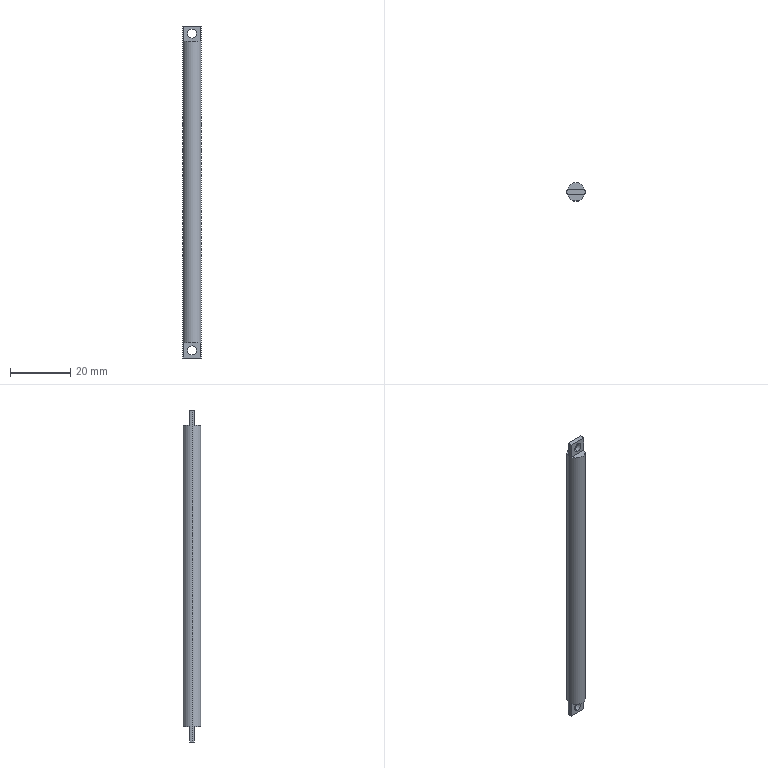Part | SolidWorks | features ICE 4, Extrusion 1 | 1 solid | 16 faces | box 6 x 6 x 110 mm | volume 2900 mm3 | plane 10 | cylinder 6 | commonest cylinder face diameters 3 x4 6 x2
STEP:
#1=CARTESIAN_POINT('',(0.,-0.8,101.));
#2=VERTEX_POINT('',#1);
#3=CARTESIAN_POINT('',(0.,-0.8,104.));
#4=VERTEX_POINT('',#3);
#5=CARTESIAN_POINT('',(0.,-0.8,102.5));
#6=DIRECTION('',(0.,1.,0.));
#7=DIRECTION('',(0.,0.,1.));
#8=AXIS2_PLACEMENT_3D('',#5,#6,#7);
#9=CIRCLE('',#8,1.5);
#10=EDGE_CURVE('',#2,#4,#9,.T.);
#11=ORIENTED_EDGE('',*,*,#10,.F.);
#12=CARTESIAN_POINT('',(0.,0.8,101.));
#13=VERTEX_POINT('',#12);
#14=CARTESIAN_POINT('',(0.,-4.2,101.));
#15=DIRECTION('',(0.,1.,0.));
#16=VECTOR('',#15,1000.);
#17=LINE('',#14,#16);
#18=EDGE_CURVE('',#2,#13,#17,.T.);
#19=ORIENTED_EDGE('',*,*,#18,.T.);
#20=CARTESIAN_POINT('',(0.,0.8,104.));
#21=VERTEX_POINT('',#20);
#22=CARTESIAN_POINT('',(0.,0.8,102.5));
#23=DIRECTION('',(0.,1.,0.));
#24=DIRECTION('',(0.,0.,1.));
#25=AXIS2_PLACEMENT_3D('',#22,#23,#24);
#26=CIRCLE('',#25,1.5);
#27=EDGE_CURVE('',#13,#21,#26,.T.);
#28=ORIENTED_EDGE('',*,*,#27,.T.);
#29=CARTESIAN_POINT('',(0.,-4.2,104.));
#30=DIRECTION('',(0.,1.,0.));
#31=VECTOR('',#30,1000.);
#32=LINE('',#29,#31);
#33=EDGE_CURVE('',#4,#21,#32,.T.);
#34=ORIENTED_EDGE('',*,*,#33,.F.);
#35=EDGE_LOOP('',(#11,#19,#28,#34));
#36=FACE_OUTER_BOUND('',#35,.T.);
#37=CARTESIAN_POINT('',(0.,-4.2,102.5));
#38=DIRECTION('',(0.,1.,0.));
#39=DIRECTION('',(0.,0.,1.));
#40=AXIS2_PLACEMENT_3D('',#37,#38,#39);
#41=CYLINDRICAL_SURFACE('',#40,1.5);
#42=ADVANCED_FACE('',(#36),#41,.F.);
#43=CARTESIAN_POINT('',(0.,-0.8,-4.));
#44=VERTEX_POINT('',#43);
#45=CARTESIAN_POINT('',(0.,-0.8,-1.));
#46=VERTEX_POINT('',#45);
#47=CARTESIAN_POINT('',(0.,-0.8,-2.5));
#48=DIRECTION('',(0.,1.,0.));
#49=DIRECTION('',(0.,0.,1.));
#50=AXIS2_PLACEMENT_3D('',#47,#48,#49);
#51=CIRCLE('',#50,1.5);
#52=EDGE_CURVE('',#44,#46,#51,.T.);
#53=ORIENTED_EDGE('',*,*,#52,.F.);
#54=CARTESIAN_POINT('',(0.,0.8,-4.));
#55=VERTEX_POINT('',#54);
#56=CARTESIAN_POINT('',(0.,-4.2,-4.));
#57=DIRECTION('',(0.,1.,0.));
#58=VECTOR('',#57,1000.);
#59=LINE('',#56,#58);
#60=EDGE_CURVE('',#44,#55,#59,.T.);
#61=ORIENTED_EDGE('',*,*,#60,.T.);
#62=CARTESIAN_POINT('',(0.,0.8,-1.));
#63=VERTEX_POINT('',#62);
#64=CARTESIAN_POINT('',(0.,0.8,-2.5));
#65=DIRECTION('',(0.,1.,0.));
#66=DIRECTION('',(0.,0.,1.));
#67=AXIS2_PLACEMENT_3D('',#64,#65,#66);
#68=CIRCLE('',#67,1.5);
#69=EDGE_CURVE('',#55,#63,#68,.T.);
#70=ORIENTED_EDGE('',*,*,#69,.T.);
#71=CARTESIAN_POINT('',(0.,-4.2,-1.));
#72=DIRECTION('',(0.,1.,0.));
#73=VECTOR('',#72,1000.);
#74=LINE('',#71,#73);
#75=EDGE_CURVE('',#46,#63,#74,.T.);
#76=ORIENTED_EDGE('',*,*,#75,.F.);
#77=EDGE_LOOP('',(#53,#61,#70,#76));
#78=FACE_OUTER_BOUND('',#77,.T.);
#79=CARTESIAN_POINT('',(0.,-4.2,-2.5));
#80=DIRECTION('',(0.,1.,0.));
#81=DIRECTION('',(0.,0.,1.));
#82=AXIS2_PLACEMENT_3D('',#79,#80,#81);
#83=CYLINDRICAL_SURFACE('',#82,1.5);
#84=ADVANCED_FACE('',(#78),#83,.F.);
#85=CARTESIAN_POINT('',(3.,0.,105.));
#86=VERTEX_POINT('',#85);
#87=CARTESIAN_POINT('',(2.891,0.8,105.));
#88=VERTEX_POINT('',#87);
#89=CARTESIAN_POINT('',(0.,0.,105.));
#90=DIRECTION('',(0.,0.,1.));
#91=DIRECTION('',(1.,0.,0.));
#92=AXIS2_PLACEMENT_3D('',#89,#90,#91);
#93=CIRCLE('',#92,3.);
#94=EDGE_CURVE('',#86,#88,#93,.T.);
#95=ORIENTED_EDGE('',*,*,#94,.F.);
#96=CARTESIAN_POINT('',(3.,0.,-5.));
#97=VERTEX_POINT('',#96);
#98=CARTESIAN_POINT('',(3.,0.,100.));
#99=DIRECTION('',(0.,0.,-1.));
#100=VECTOR('',#99,1000.);
#101=LINE('',#98,#100);
#102=EDGE_CURVE('',#86,#97,#101,.T.);
#103=ORIENTED_EDGE('',*,*,#102,.T.);
#104=CARTESIAN_POINT('',(2.891,0.8,-5.));
#105=VERTEX_POINT('',#104);
#106=CARTESIAN_POINT('',(0.,0.,-5.));
#107=DIRECTION('',(0.,0.,-1.));
#108=DIRECTION('',(-1.,0.,0.));
#109=AXIS2_PLACEMENT_3D('',#106,#107,#108);
#110=CIRCLE('',#109,3.);
#111=EDGE_CURVE('',#105,#97,#110,.T.);
#112=ORIENTED_EDGE('',*,*,#111,.F.);
#113=CARTESIAN_POINT('',(2.891,0.8,0.));
#114=VERTEX_POINT('',#113);
#115=CARTESIAN_POINT('',(2.891,0.8,-5.));
#116=DIRECTION('',(0.,0.,1.));
#117=VECTOR('',#116,1000.);
#118=LINE('',#115,#117);
#119=EDGE_CURVE('',#105,#114,#118,.T.);
#120=ORIENTED_EDGE('',*,*,#119,.T.);
#121=CARTESIAN_POINT('',(-2.891,0.8,0.));
#122=VERTEX_POINT('',#121);
#123=CARTESIAN_POINT('',(0.,0.,0.));
#124=DIRECTION('',(0.,0.,1.));
#125=DIRECTION('',(1.,0.,0.));
#126=AXIS2_PLACEMENT_3D('',#123,#124,#125);
#127=CIRCLE('',#126,3.);
#128=EDGE_CURVE('',#114,#122,#127,.T.);
#129=ORIENTED_EDGE('',*,*,#128,.T.);
#130=CARTESIAN_POINT('',(-2.891,0.8,-5.));
#131=VERTEX_POINT('',#130);
#132=CARTESIAN_POINT('',(-2.891,0.8,-5.));
#133=DIRECTION('',(0.,0.,1.));
#134=VECTOR('',#133,1000.);
#135=LINE('',#132,#134);
#136=EDGE_CURVE('',#131,#122,#135,.T.);
#137=ORIENTED_EDGE('',*,*,#136,.F.);
#138=CARTESIAN_POINT('',(-3.,0.,-5.));
#139=VERTEX_POINT('',#138);
#140=CARTESIAN_POINT('',(0.,0.,-5.));
#141=DIRECTION('',(0.,0.,-1.));
#142=DIRECTION('',(-1.,0.,0.));
#143=AXIS2_PLACEMENT_3D('',#140,#141,#142);
#144=CIRCLE('',#143,3.);
#145=EDGE_CURVE('',#139,#131,#144,.T.);
#146=ORIENTED_EDGE('',*,*,#145,.F.);
#147=CARTESIAN_POINT('',(-3.,0.,105.));
#148=VERTEX_POINT('',#147);
#149=CARTESIAN_POINT('',(-3.,0.,100.));
#150=DIRECTION('',(0.,0.,-1.));
#151=VECTOR('',#150,1000.);
#152=LINE('',#149,#151);
#153=EDGE_CURVE('',#148,#139,#152,.T.);
#154=ORIENTED_EDGE('',*,*,#153,.F.);
#155=CARTESIAN_POINT('',(-2.891,0.8,105.));
#156=VERTEX_POINT('',#155);
#157=CARTESIAN_POINT('',(0.,0.,105.));
#158=DIRECTION('',(0.,0.,1.));
#159=DIRECTION('',(1.,0.,0.));
#160=AXIS2_PLACEMENT_3D('',#157,#158,#159);
#161=CIRCLE('',#160,3.);
#162=EDGE_CURVE('',#156,#148,#161,.T.);
#163=ORIENTED_EDGE('',*,*,#162,.F.);
#164=CARTESIAN_POINT('',(-2.891,0.8,100.));
#165=VERTEX_POINT('',#164);
#166=CARTESIAN_POINT('',(-2.891,0.8,105.));
#167=DIRECTION('',(0.,0.,-1.));
#168=VECTOR('',#167,1000.);
#169=LINE('',#166,#168);
#170=EDGE_CURVE('',#156,#165,#169,.T.);
#171=ORIENTED_EDGE('',*,*,#170,.T.);
#172=CARTESIAN_POINT('',(2.891,0.8,100.));
#173=VERTEX_POINT('',#172);
#174=CARTESIAN_POINT('',(0.,0.,100.));
#175=DIRECTION('',(0.,0.,1.));
#176=DIRECTION('',(1.,0.,0.));
#177=AXIS2_PLACEMENT_3D('',#174,#175,#176);
#178=CIRCLE('',#177,3.);
#179=EDGE_CURVE('',#173,#165,#178,.T.);
#180=ORIENTED_EDGE('',*,*,#179,.F.);
#181=CARTESIAN_POINT('',(2.891,0.8,105.));
#182=DIRECTION('',(0.,0.,-1.));
#183=VECTOR('',#182,1000.);
#184=LINE('',#181,#183);
#185=EDGE_CURVE('',#88,#173,#184,.T.);
#186=ORIENTED_EDGE('',*,*,#185,.F.);
#187=EDGE_LOOP('',(#95,#103,#112,#120,#129,#137,#146,#154,#163,#171,#180,#186));
#188=FACE_OUTER_BOUND('',#187,.T.);
#189=CARTESIAN_POINT('',(0.,0.,100.));
#190=DIRECTION('',(0.,0.,-1.));
#191=DIRECTION('',(-1.,0.,0.));
#192=AXIS2_PLACEMENT_3D('',#189,#190,#191);
#193=CYLINDRICAL_SURFACE('',#192,3.);
#194=ADVANCED_FACE('',(#188),#193,.T.);
#195=CARTESIAN_POINT('',(2.891,0.8,0.));
#196=DIRECTION('',(1.,0.,0.));
#197=VECTOR('',#196,1000.);
#198=LINE('',#195,#197);
#199=EDGE_CURVE('',#122,#114,#198,.T.);
#200=ORIENTED_EDGE('',*,*,#199,.F.);
#201=ORIENTED_EDGE('',*,*,#128,.F.);
#202=EDGE_LOOP('',(#200,#201));
#203=FACE_OUTER_BOUND('',#202,.T.);
#204=CARTESIAN_POINT('',(0.,0.,0.));
#205=DIRECTION('',(0.,0.,1.));
#206=DIRECTION('',(1.,0.,0.));
#207=AXIS2_PLACEMENT_3D('',#204,#205,#206);
#208=PLANE('',#207);
#209=ADVANCED_FACE('',(#203),#208,.F.);
#210=CARTESIAN_POINT('',(2.891,-0.8,0.));
#211=VERTEX_POINT('',#210);
#212=CARTESIAN_POINT('',(-2.891,-0.8,0.));
#213=VERTEX_POINT('',#212);
#214=CARTESIAN_POINT('',(2.891,-0.8,0.));
#215=DIRECTION('',(-1.,0.,0.));
#216=VECTOR('',#215,1000.);
#217=LINE('',#214,#216);
#218=EDGE_CURVE('',#211,#213,#217,.T.);
#219=ORIENTED_EDGE('',*,*,#218,.F.);
#220=CARTESIAN_POINT('',(0.,0.,0.));
#221=DIRECTION('',(0.,0.,1.));
#222=DIRECTION('',(1.,0.,0.));
#223=AXIS2_PLACEMENT_3D('',#220,#221,#222);
#224=CIRCLE('',#223,3.);
#225=EDGE_CURVE('',#213,#211,#224,.T.);
#226=ORIENTED_EDGE('',*,*,#225,.F.);
#227=EDGE_LOOP('',(#219,#226));
#228=FACE_OUTER_BOUND('',#227,.T.);
#229=CARTESIAN_POINT('',(0.,0.,0.));
#230=DIRECTION('',(0.,0.,1.));
#231=DIRECTION('',(1.,0.,0.));
#232=AXIS2_PLACEMENT_3D('',#229,#230,#231);
#233=PLANE('',#232);
#234=ADVANCED_FACE('',(#228),#233,.F.);
#235=CARTESIAN_POINT('',(-2.891,0.8,100.));
#236=DIRECTION('',(-1.,0.,0.));
#237=VECTOR('',#236,1000.);
#238=LINE('',#235,#237);
#239=EDGE_CURVE('',#173,#165,#238,.T.);
#240=ORIENTED_EDGE('',*,*,#239,.F.);
#241=ORIENTED_EDGE('',*,*,#179,.T.);
#242=EDGE_LOOP('',(#240,#241));
#243=FACE_OUTER_BOUND('',#242,.T.);
#244=CARTESIAN_POINT('',(0.,0.,100.));
#245=DIRECTION('',(0.,0.,1.));
#246=DIRECTION('',(1.,0.,0.));
#247=AXIS2_PLACEMENT_3D('',#244,#245,#246);
#248=PLANE('',#247);
#249=ADVANCED_FACE('',(#243),#248,.T.);
#250=ORIENTED_EDGE('',*,*,#102,.F.);
#251=CARTESIAN_POINT('',(2.891,-0.8,105.));
#252=VERTEX_POINT('',#251);
#253=CARTESIAN_POINT('',(0.,0.,105.));
#254=DIRECTION('',(0.,0.,1.));
#255=DIRECTION('',(1.,0.,0.));
#256=AXIS2_PLACEMENT_3D('',#253,#254,#255);
#257=CIRCLE('',#256,3.);
#258=EDGE_CURVE('',#252,#86,#257,.T.);
#259=ORIENTED_EDGE('',*,*,#258,.F.);
#260=CARTESIAN_POINT('',(2.891,-0.8,100.));
#261=VERTEX_POINT('',#260);
#262=CARTESIAN_POINT('',(2.891,-0.8,105.));
#263=DIRECTION('',(0.,0.,-1.));
#264=VECTOR('',#263,1000.);
#265=LINE('',#262,#264);
#266=EDGE_CURVE('',#252,#261,#265,.T.);
#267=ORIENTED_EDGE('',*,*,#266,.T.);
#268=CARTESIAN_POINT('',(-2.891,-0.8,100.));
#269=VERTEX_POINT('',#268);
#270=CARTESIAN_POINT('',(0.,0.,100.));
#271=DIRECTION('',(0.,0.,1.));
#272=DIRECTION('',(1.,0.,0.));
#273=AXIS2_PLACEMENT_3D('',#270,#271,#272);
#274=CIRCLE('',#273,3.);
#275=EDGE_CURVE('',#269,#261,#274,.T.);
#276=ORIENTED_EDGE('',*,*,#275,.F.);
#277=CARTESIAN_POINT('',(-2.891,-0.8,105.));
#278=VERTEX_POINT('',#277);
#279=CARTESIAN_POINT('',(-2.891,-0.8,105.));
#280=DIRECTION('',(0.,0.,-1.));
#281=VECTOR('',#280,1000.);
#282=LINE('',#279,#281);
#283=EDGE_CURVE('',#278,#269,#282,.T.);
#284=ORIENTED_EDGE('',*,*,#283,.F.);
#285=CARTESIAN_POINT('',(0.,0.,105.));
#286=DIRECTION('',(0.,0.,1.));
#287=DIRECTION('',(1.,0.,0.));
#288=AXIS2_PLACEMENT_3D('',#285,#286,#287);
#289=CIRCLE('',#288,3.);
#290=EDGE_CURVE('',#148,#278,#289,.T.);
#291=ORIENTED_EDGE('',*,*,#290,.F.);
#292=ORIENTED_EDGE('',*,*,#153,.T.);
#293=CARTESIAN_POINT('',(-2.891,-0.8,-5.));
#294=VERTEX_POINT('',#293);
#295=CARTESIAN_POINT('',(0.,0.,-5.));
#296=DIRECTION('',(0.,0.,-1.));
#297=DIRECTION('',(-1.,0.,0.));
#298=AXIS2_PLACEMENT_3D('',#295,#296,#297);
#299=CIRCLE('',#298,3.);
#300=EDGE_CURVE('',#294,#139,#299,.T.);
#301=ORIENTED_EDGE('',*,*,#300,.F.);
#302=CARTESIAN_POINT('',(-2.891,-0.8,-5.));
#303=DIRECTION('',(0.,0.,1.));
#304=VECTOR('',#303,1000.);
#305=LINE('',#302,#304);
#306=EDGE_CURVE('',#294,#213,#305,.T.);
#307=ORIENTED_EDGE('',*,*,#306,.T.);
#308=ORIENTED_EDGE('',*,*,#225,.T.);
#309=CARTESIAN_POINT('',(2.891,-0.8,-5.));
#310=VERTEX_POINT('',#309);
#311=CARTESIAN_POINT('',(2.891,-0.8,-5.));
#312=DIRECTION('',(0.,0.,1.));
#313=VECTOR('',#312,1000.);
#314=LINE('',#311,#313);
#315=EDGE_CURVE('',#310,#211,#314,.T.);
#316=ORIENTED_EDGE('',*,*,#315,.F.);
#317=CARTESIAN_POINT('',(0.,0.,-5.));
#318=DIRECTION('',(0.,0.,-1.));
#319=DIRECTION('',(-1.,0.,0.));
#320=AXIS2_PLACEMENT_3D('',#317,#318,#319);
#321=CIRCLE('',#320,3.);
#322=EDGE_CURVE('',#97,#310,#321,.T.);
#323=ORIENTED_EDGE('',*,*,#322,.F.);
#324=EDGE_LOOP('',(#250,#259,#267,#276,#284,#291,#292,#301,#307,#308,#316,#323));
#325=FACE_OUTER_BOUND('',#324,.T.);
#326=CARTESIAN_POINT('',(0.,0.,100.));
#327=DIRECTION('',(0.,0.,-1.));
#328=DIRECTION('',(-1.,0.,0.));
#329=AXIS2_PLACEMENT_3D('',#326,#327,#328);
#330=CYLINDRICAL_SURFACE('',#329,3.);
#331=ADVANCED_FACE('',(#325),#330,.T.);
#332=CARTESIAN_POINT('',(-2.891,-0.8,100.));
#333=DIRECTION('',(1.,0.,0.));
#334=VECTOR('',#333,1000.);
#335=LINE('',#332,#334);
#336=EDGE_CURVE('',#269,#261,#335,.T.);
#337=ORIENTED_EDGE('',*,*,#336,.F.);
#338=ORIENTED_EDGE('',*,*,#275,.T.);
#339=EDGE_LOOP('',(#337,#338));
#340=FACE_OUTER_BOUND('',#339,.T.);
#341=CARTESIAN_POINT('',(0.,0.,100.));
#342=DIRECTION('',(0.,0.,1.));
#343=DIRECTION('',(1.,0.,0.));
#344=AXIS2_PLACEMENT_3D('',#341,#342,#343);
#345=PLANE('',#344);
#346=ADVANCED_FACE('',(#340),#345,.T.);
#347=CARTESIAN_POINT('',(0.,-0.8,102.5));
#348=DIRECTION('',(0.,1.,0.));
#349=DIRECTION('',(0.,0.,1.));
#350=AXIS2_PLACEMENT_3D('',#347,#348,#349);
#351=CIRCLE('',#350,1.5);
#352=EDGE_CURVE('',#4,#2,#351,.T.);
#353=ORIENTED_EDGE('',*,*,#352,.T.);
#354=ORIENTED_EDGE('',*,*,#10,.T.);
#355=EDGE_LOOP('',(#353,#354));
#356=FACE_BOUND('',#355,.T.);
#357=ORIENTED_EDGE('',*,*,#336,.T.);
#358=ORIENTED_EDGE('',*,*,#266,.F.);
#359=CARTESIAN_POINT('',(-2.891,-0.8,105.));
#360=DIRECTION('',(1.,0.,0.));
#361=VECTOR('',#360,1000.);
#362=LINE('',#359,#361);
#363=EDGE_CURVE('',#278,#252,#362,.T.);
#364=ORIENTED_EDGE('',*,*,#363,.F.);
#365=ORIENTED_EDGE('',*,*,#283,.T.);
#366=EDGE_LOOP('',(#357,#358,#364,#365));
#367=FACE_OUTER_BOUND('',#366,.T.);
#368=CARTESIAN_POINT('',(-2.891,-0.8,105.));
#369=DIRECTION('',(0.,1.,0.));
#370=DIRECTION('',(0.,0.,1.));
#371=AXIS2_PLACEMENT_3D('',#368,#369,#370);
#372=PLANE('',#371);
#373=ADVANCED_FACE('',(#356,#367),#372,.F.);
#374=CARTESIAN_POINT('',(0.,0.8,102.5));
#375=DIRECTION('',(0.,1.,0.));
#376=DIRECTION('',(0.,0.,1.));
#377=AXIS2_PLACEMENT_3D('',#374,#375,#376);
#378=CIRCLE('',#377,1.5);
#379=EDGE_CURVE('',#21,#13,#378,.T.);
#380=ORIENTED_EDGE('',*,*,#379,.F.);
#381=ORIENTED_EDGE('',*,*,#27,.F.);
#382=EDGE_LOOP('',(#380,#381));
#383=FACE_BOUND('',#382,.T.);
#384=ORIENTED_EDGE('',*,*,#239,.T.);
#385=ORIENTED_EDGE('',*,*,#170,.F.);
#386=CARTESIAN_POINT('',(-2.891,0.8,105.));
#387=DIRECTION('',(-1.,0.,0.));
#388=VECTOR('',#387,1000.);
#389=LINE('',#386,#388);
#390=EDGE_CURVE('',#88,#156,#389,.T.);
#391=ORIENTED_EDGE('',*,*,#390,.F.);
#392=ORIENTED_EDGE('',*,*,#185,.T.);
#393=EDGE_LOOP('',(#384,#385,#391,#392));
#394=FACE_OUTER_BOUND('',#393,.T.);
#395=CARTESIAN_POINT('',(-2.891,0.8,105.));
#396=DIRECTION('',(0.,-1.,0.));
#397=DIRECTION('',(0.,0.,-1.));
#398=AXIS2_PLACEMENT_3D('',#395,#396,#397);
#399=PLANE('',#398);
#400=ADVANCED_FACE('',(#383,#394),#399,.F.);
#401=ORIENTED_EDGE('',*,*,#162,.T.);
#402=ORIENTED_EDGE('',*,*,#290,.T.);
#403=ORIENTED_EDGE('',*,*,#363,.T.);
#404=ORIENTED_EDGE('',*,*,#258,.T.);
#405=ORIENTED_EDGE('',*,*,#94,.T.);
#406=ORIENTED_EDGE('',*,*,#390,.T.);
#407=EDGE_LOOP('',(#401,#402,#403,#404,#405,#406));
#408=FACE_OUTER_BOUND('',#407,.T.);
#409=CARTESIAN_POINT('',(0.,0.,105.));
#410=DIRECTION('',(0.,0.,1.));
#411=DIRECTION('',(1.,0.,0.));
#412=AXIS2_PLACEMENT_3D('',#409,#410,#411);
#413=PLANE('',#412);
#414=ADVANCED_FACE('',(#408),#413,.T.);
#415=CARTESIAN_POINT('',(0.,-0.8,-2.5));
#416=DIRECTION('',(0.,1.,0.));
#417=DIRECTION('',(0.,0.,1.));
#418=AXIS2_PLACEMENT_3D('',#415,#416,#417);
#419=CIRCLE('',#418,1.5);
#420=EDGE_CURVE('',#46,#44,#419,.T.);
#421=ORIENTED_EDGE('',*,*,#420,.T.);
#422=ORIENTED_EDGE('',*,*,#52,.T.);
#423=EDGE_LOOP('',(#421,#422));
#424=FACE_BOUND('',#423,.T.);
#425=ORIENTED_EDGE('',*,*,#218,.T.);
#426=ORIENTED_EDGE('',*,*,#306,.F.);
#427=CARTESIAN_POINT('',(2.891,-0.8,-5.));
#428=DIRECTION('',(-1.,0.,0.));
#429=VECTOR('',#428,1000.);
#430=LINE('',#427,#429);
#431=EDGE_CURVE('',#310,#294,#430,.T.);
#432=ORIENTED_EDGE('',*,*,#431,.F.);
#433=ORIENTED_EDGE('',*,*,#315,.T.);
#434=EDGE_LOOP('',(#425,#426,#432,#433));
#435=FACE_OUTER_BOUND('',#434,.T.);
#436=CARTESIAN_POINT('',(2.891,-0.8,-5.));
#437=DIRECTION('',(0.,1.,0.));
#438=DIRECTION('',(0.,0.,1.));
#439=AXIS2_PLACEMENT_3D('',#436,#437,#438);
#440=PLANE('',#439);
#441=ADVANCED_FACE('',(#424,#435),#440,.F.);
#442=CARTESIAN_POINT('',(0.,0.8,-2.5));
#443=DIRECTION('',(0.,1.,0.));
#444=DIRECTION('',(0.,0.,1.));
#445=AXIS2_PLACEMENT_3D('',#442,#443,#444);
#446=CIRCLE('',#445,1.5);
#447=EDGE_CURVE('',#63,#55,#446,.T.);
#448=ORIENTED_EDGE('',*,*,#447,.F.);
#449=ORIENTED_EDGE('',*,*,#69,.F.);
#450=EDGE_LOOP('',(#448,#449));
#451=FACE_BOUND('',#450,.T.);
#452=ORIENTED_EDGE('',*,*,#199,.T.);
#453=ORIENTED_EDGE('',*,*,#119,.F.);
#454=CARTESIAN_POINT('',(2.891,0.8,-5.));
#455=DIRECTION('',(1.,0.,0.));
#456=VECTOR('',#455,1000.);
#457=LINE('',#454,#456);
#458=EDGE_CURVE('',#131,#105,#457,.T.);
#459=ORIENTED_EDGE('',*,*,#458,.F.);
#460=ORIENTED_EDGE('',*,*,#136,.T.);
#461=EDGE_LOOP('',(#452,#453,#459,#460));
#462=FACE_OUTER_BOUND('',#461,.T.);
#463=CARTESIAN_POINT('',(2.891,0.8,-5.));
#464=DIRECTION('',(0.,-1.,0.));
#465=DIRECTION('',(0.,0.,-1.));
#466=AXIS2_PLACEMENT_3D('',#463,#464,#465);
#467=PLANE('',#466);
#468=ADVANCED_FACE('',(#451,#462),#467,.F.);
#469=ORIENTED_EDGE('',*,*,#111,.T.);
#470=ORIENTED_EDGE('',*,*,#322,.T.);
#471=ORIENTED_EDGE('',*,*,#431,.T.);
#472=ORIENTED_EDGE('',*,*,#300,.T.);
#473=ORIENTED_EDGE('',*,*,#145,.T.);
#474=ORIENTED_EDGE('',*,*,#458,.T.);
#475=EDGE_LOOP('',(#469,#470,#471,#472,#473,#474));
#476=FACE_OUTER_BOUND('',#475,.T.);
#477=CARTESIAN_POINT('',(0.,0.,-5.));
#478=DIRECTION('',(0.,0.,-1.));
#479=DIRECTION('',(-1.,0.,0.));
#480=AXIS2_PLACEMENT_3D('',#477,#478,#479);
#481=PLANE('',#480);
#482=ADVANCED_FACE('',(#476),#481,.T.);
#483=ORIENTED_EDGE('',*,*,#60,.F.);
#484=ORIENTED_EDGE('',*,*,#420,.F.);
#485=ORIENTED_EDGE('',*,*,#75,.T.);
#486=ORIENTED_EDGE('',*,*,#447,.T.);
#487=EDGE_LOOP('',(#483,#484,#485,#486));
#488=FACE_OUTER_BOUND('',#487,.T.);
#489=CARTESIAN_POINT('',(0.,-4.2,-2.5));
#490=DIRECTION('',(0.,1.,0.));
#491=DIRECTION('',(0.,0.,1.));
#492=AXIS2_PLACEMENT_3D('',#489,#490,#491);
#493=CYLINDRICAL_SURFACE('',#492,1.5);
#494=ADVANCED_FACE('',(#488),#493,.F.);
#495=ORIENTED_EDGE('',*,*,#18,.F.);
#496=ORIENTED_EDGE('',*,*,#352,.F.);
#497=ORIENTED_EDGE('',*,*,#33,.T.);
#498=ORIENTED_EDGE('',*,*,#379,.T.);
#499=EDGE_LOOP('',(#495,#496,#497,#498));
#500=FACE_OUTER_BOUND('',#499,.T.);
#501=CARTESIAN_POINT('',(0.,-4.2,102.5));
#502=DIRECTION('',(0.,1.,0.));
#503=DIRECTION('',(0.,0.,1.));
#504=AXIS2_PLACEMENT_3D('',#501,#502,#503);
#505=CYLINDRICAL_SURFACE('',#504,1.5);
#506=ADVANCED_FACE('',(#500),#505,.F.);
#507=CLOSED_SHELL('',(#42,#84,#194,#209,#234,#249,#331,#346,#373,#400,#414,#441,#468,#482,#494,#506));
#508=MANIFOLD_SOLID_BREP('',#507);
#509=CARTESIAN_POINT('',(0.,0.,0.));
#510=DIRECTION('',(0.,0.,1.));
#511=DIRECTION('',(1.,0.,0.));
#512=AXIS2_PLACEMENT_3D('',#509,#510,#511);
#513=(LENGTH_UNIT()NAMED_UNIT(*)SI_UNIT(.MILLI.,.METRE.));
#514=UNCERTAINTY_MEASURE_WITH_UNIT(LENGTH_MEASURE(0.00001),#513,'','');
#515=(NAMED_UNIT(*)PLANE_ANGLE_UNIT()SI_UNIT($,.RADIAN.));
#516=(NAMED_UNIT(*)SI_UNIT($,.STERADIAN.)SOLID_ANGLE_UNIT());
#517=(GEOMETRIC_REPRESENTATION_CONTEXT(3)GLOBAL_UNCERTAINTY_ASSIGNED_CONTEXT((#514))GLOBAL_UNIT_ASSIGNED_CONTEXT((#513,#515,#516))REPRESENTATION_CONTEXT('',''));
#518=ADVANCED_BREP_SHAPE_REPRESENTATION('',(#508,#512),#517);